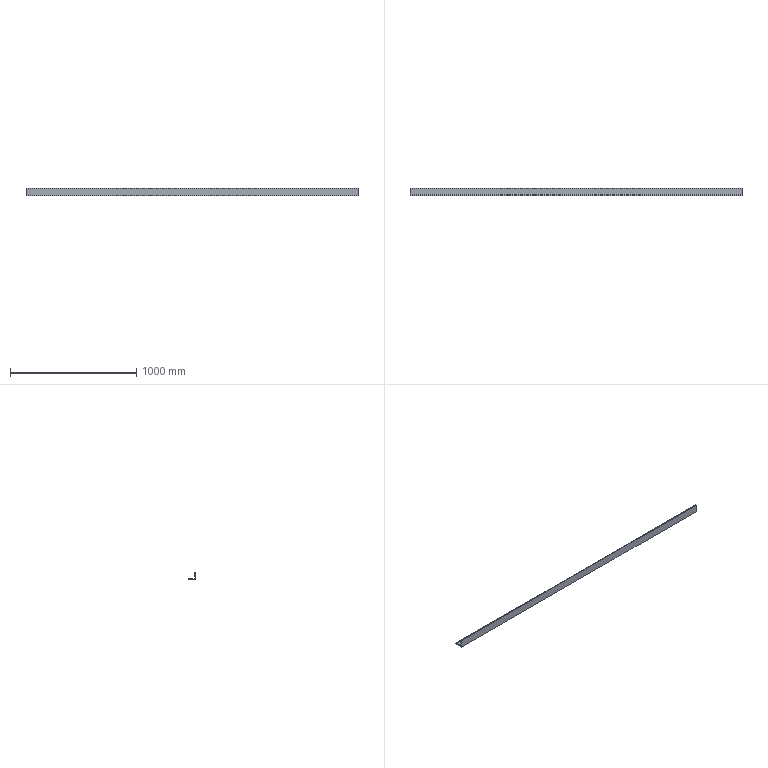Part | STEP file | Angle steel L63X63X8-2626_Default<As machined> | 1 solid | 11 faces | box 2626 x 63 x 63 mm | volume 2498543 mm3 | plane 8 | cylinder 3 | commonest cylinder face diameters 5.333 x2 14 x1
STEP:
#1=CARTESIAN_POINT('',(0.,0.,0.));
#2=DIRECTION('',(0.,0.,1.));
#3=DIRECTION('',(1.,0.,0.));
#4=AXIS2_PLACEMENT_3D('',#1,#2,#3);
#5=CARTESIAN_POINT('',(-1313.,0.,0.));
#6=VERTEX_POINT('',#5);
#7=CARTESIAN_POINT('',(-1313.,63.,0.));
#8=VERTEX_POINT('',#7);
#9=CARTESIAN_POINT('',(-1313.,63.,0.));
#10=DIRECTION('',(0.,1.,0.));
#11=VECTOR('',#10,1.);
#12=LINE('',#9,#11);
#13=CARTESIAN_POINT('',(1313.,63.,0.));
#14=DIRECTION('',(0.,0.,1.));
#15=DIRECTION('',(1.,0.,0.));
#16=AXIS2_PLACEMENT_3D('',#13,#14,#15);
#17=PLANE('',#16);
#18=CARTESIAN_POINT('',(-2626.,0.));
#19=DIRECTION('',(0.,1.));
#20=VECTOR('',#19,1.);
#21=LINE('',#18,#20);
#22=(GEOMETRIC_REPRESENTATION_CONTEXT(2)PARAMETRIC_REPRESENTATION_CONTEXT()REPRESENTATION_CONTEXT('',''));
#23=DEFINITIONAL_REPRESENTATION('',(#21),#22);
#24=PCURVE('',#17,#23);
#25=CARTESIAN_POINT('',(-1313.,5.333,60.333));
#26=DIRECTION('',(-1.,0.,0.));
#27=DIRECTION('',(0.,0.,1.));
#28=AXIS2_PLACEMENT_3D('',#25,#26,#27);
#29=PLANE('',#28);
#30=CARTESIAN_POINT('',(-60.333,57.667));
#31=DIRECTION('',(0.,1.));
#32=VECTOR('',#31,1.);
#33=LINE('',#30,#32);
#34=(GEOMETRIC_REPRESENTATION_CONTEXT(2)PARAMETRIC_REPRESENTATION_CONTEXT()REPRESENTATION_CONTEXT('',''));
#35=DEFINITIONAL_REPRESENTATION('',(#33),#34);
#36=PCURVE('',#29,#35);
#37=SURFACE_CURVE('',#12,(#24,#36),.PCURVE_S1.);
#38=EDGE_CURVE('',#6,#8,#37,.T.);
#39=ORIENTED_EDGE('',*,*,#38,.T.);
#40=CARTESIAN_POINT('',(1313.,63.,0.));
#41=VERTEX_POINT('',#40);
#42=CARTESIAN_POINT('',(1313.,63.,0.));
#43=DIRECTION('',(-1.,0.,0.));
#44=VECTOR('',#43,1.);
#45=LINE('',#42,#44);
#46=CARTESIAN_POINT('',(0.,0.));
#47=DIRECTION('',(-1.,0.));
#48=VECTOR('',#47,1.);
#49=LINE('',#46,#48);
#50=(GEOMETRIC_REPRESENTATION_CONTEXT(2)PARAMETRIC_REPRESENTATION_CONTEXT()REPRESENTATION_CONTEXT('',''));
#51=DEFINITIONAL_REPRESENTATION('',(#49),#50);
#52=PCURVE('',#17,#51);
#53=CARTESIAN_POINT('',(1313.,63.,0.));
#54=DIRECTION('',(0.,-1.,0.));
#55=DIRECTION('',(0.,0.,-1.));
#56=AXIS2_PLACEMENT_3D('',#53,#54,#55);
#57=PLANE('',#56);
#58=CARTESIAN_POINT('',(0.,0.));
#59=DIRECTION('',(0.,-1.));
#60=VECTOR('',#59,1.);
#61=LINE('',#58,#60);
#62=(GEOMETRIC_REPRESENTATION_CONTEXT(2)PARAMETRIC_REPRESENTATION_CONTEXT()REPRESENTATION_CONTEXT('',''));
#63=DEFINITIONAL_REPRESENTATION('',(#61),#62);
#64=PCURVE('',#57,#63);
#65=SURFACE_CURVE('',#45,(#52,#64),.PCURVE_S1.);
#66=EDGE_CURVE('',#41,#8,#65,.T.);
#67=ORIENTED_EDGE('',*,*,#66,.F.);
#68=CARTESIAN_POINT('',(1313.,0.,0.));
#69=VERTEX_POINT('',#68);
#70=CARTESIAN_POINT('',(1313.,63.,0.));
#71=DIRECTION('',(0.,1.,0.));
#72=VECTOR('',#71,1.);
#73=LINE('',#70,#72);
#74=CARTESIAN_POINT('',(0.,0.));
#75=DIRECTION('',(0.,1.));
#76=VECTOR('',#75,1.);
#77=LINE('',#74,#76);
#78=(GEOMETRIC_REPRESENTATION_CONTEXT(2)PARAMETRIC_REPRESENTATION_CONTEXT()REPRESENTATION_CONTEXT('',''));
#79=DEFINITIONAL_REPRESENTATION('',(#77),#78);
#80=PCURVE('',#17,#79);
#81=CARTESIAN_POINT('',(1313.,5.333,60.333));
#82=DIRECTION('',(-1.,0.,0.));
#83=DIRECTION('',(0.,0.,1.));
#84=AXIS2_PLACEMENT_3D('',#81,#82,#83);
#85=PLANE('',#84);
#86=CARTESIAN_POINT('',(-60.333,57.667));
#87=DIRECTION('',(0.,1.));
#88=VECTOR('',#87,1.);
#89=LINE('',#86,#88);
#90=(GEOMETRIC_REPRESENTATION_CONTEXT(2)PARAMETRIC_REPRESENTATION_CONTEXT()REPRESENTATION_CONTEXT('',''));
#91=DEFINITIONAL_REPRESENTATION('',(#89),#90);
#92=PCURVE('',#85,#91);
#93=SURFACE_CURVE('',#73,(#80,#92),.PCURVE_S1.);
#94=EDGE_CURVE('',#69,#41,#93,.T.);
#95=ORIENTED_EDGE('',*,*,#94,.F.);
#96=CARTESIAN_POINT('',(1313.,0.,0.));
#97=DIRECTION('',(-1.,0.,0.));
#98=VECTOR('',#97,1.);
#99=LINE('',#96,#98);
#100=CARTESIAN_POINT('',(0.,-63.));
#101=DIRECTION('',(-1.,0.));
#102=VECTOR('',#101,1.);
#103=LINE('',#100,#102);
#104=(GEOMETRIC_REPRESENTATION_CONTEXT(2)PARAMETRIC_REPRESENTATION_CONTEXT()REPRESENTATION_CONTEXT('',''));
#105=DEFINITIONAL_REPRESENTATION('',(#103),#104);
#106=PCURVE('',#17,#105);
#107=CARTESIAN_POINT('',(1313.,0.,0.));
#108=DIRECTION('',(0.,1.,0.));
#109=DIRECTION('',(0.,0.,1.));
#110=AXIS2_PLACEMENT_3D('',#107,#108,#109);
#111=PLANE('',#110);
#112=CARTESIAN_POINT('',(0.,0.));
#113=DIRECTION('',(0.,-1.));
#114=VECTOR('',#113,1.);
#115=LINE('',#112,#114);
#116=(GEOMETRIC_REPRESENTATION_CONTEXT(2)PARAMETRIC_REPRESENTATION_CONTEXT()REPRESENTATION_CONTEXT('',''));
#117=DEFINITIONAL_REPRESENTATION('',(#115),#116);
#118=PCURVE('',#111,#117);
#119=SURFACE_CURVE('',#99,(#106,#118),.PCURVE_S1.);
#120=EDGE_CURVE('',#69,#6,#119,.T.);
#121=ORIENTED_EDGE('',*,*,#120,.T.);
#122=EDGE_LOOP('',(#39,#67,#95,#121));
#123=FACE_BOUND('',#122,.T.);
#124=ADVANCED_FACE('',(#123),#17,.F.);
#125=CARTESIAN_POINT('',(-1313.,63.,5.333));
#126=VERTEX_POINT('',#125);
#127=CARTESIAN_POINT('',(-1313.,63.,0.));
#128=DIRECTION('',(0.,0.,1.));
#129=VECTOR('',#128,1.);
#130=LINE('',#127,#129);
#131=CARTESIAN_POINT('',(0.,-2626.));
#132=DIRECTION('',(-1.,0.));
#133=VECTOR('',#132,1.);
#134=LINE('',#131,#133);
#135=(GEOMETRIC_REPRESENTATION_CONTEXT(2)PARAMETRIC_REPRESENTATION_CONTEXT()REPRESENTATION_CONTEXT('',''));
#136=DEFINITIONAL_REPRESENTATION('',(#134),#135);
#137=PCURVE('',#57,#136);
#138=CARTESIAN_POINT('',(-60.333,57.667));
#139=DIRECTION('',(1.,0.));
#140=VECTOR('',#139,1.);
#141=LINE('',#138,#140);
#142=(GEOMETRIC_REPRESENTATION_CONTEXT(2)PARAMETRIC_REPRESENTATION_CONTEXT()REPRESENTATION_CONTEXT('',''));
#143=DEFINITIONAL_REPRESENTATION('',(#141),#142);
#144=PCURVE('',#29,#143);
#145=SURFACE_CURVE('',#130,(#137,#144),.PCURVE_S1.);
#146=EDGE_CURVE('',#8,#126,#145,.T.);
#147=ORIENTED_EDGE('',*,*,#146,.T.);
#148=CARTESIAN_POINT('',(1313.,63.,5.333));
#149=VERTEX_POINT('',#148);
#150=CARTESIAN_POINT('',(1313.,63.,5.333));
#151=DIRECTION('',(-1.,0.,0.));
#152=VECTOR('',#151,1.);
#153=LINE('',#150,#152);
#154=CARTESIAN_POINT('',(-5.333,0.));
#155=DIRECTION('',(0.,-1.));
#156=VECTOR('',#155,1.);
#157=LINE('',#154,#156);
#158=(GEOMETRIC_REPRESENTATION_CONTEXT(2)PARAMETRIC_REPRESENTATION_CONTEXT()REPRESENTATION_CONTEXT('',''));
#159=DEFINITIONAL_REPRESENTATION('',(#157),#158);
#160=PCURVE('',#57,#159);
#161=CARTESIAN_POINT('',(1313.,60.333,5.333));
#162=DIRECTION('',(-1.,0.,0.));
#163=DIRECTION('',(0.,0.,1.));
#164=AXIS2_PLACEMENT_3D('',#161,#162,#163);
#165=CYLINDRICAL_SURFACE('',#164,2.667);
#166=CARTESIAN_POINT('',(1.571,0.));
#167=DIRECTION('',(0.,1.));
#168=VECTOR('',#167,1.);
#169=LINE('',#166,#168);
#170=(GEOMETRIC_REPRESENTATION_CONTEXT(2)PARAMETRIC_REPRESENTATION_CONTEXT()REPRESENTATION_CONTEXT('',''));
#171=DEFINITIONAL_REPRESENTATION('',(#169),#170);
#172=PCURVE('',#165,#171);
#173=SURFACE_CURVE('',#153,(#160,#172),.PCURVE_S1.);
#174=EDGE_CURVE('',#149,#126,#173,.T.);
#175=ORIENTED_EDGE('',*,*,#174,.F.);
#176=CARTESIAN_POINT('',(1313.,63.,0.));
#177=DIRECTION('',(0.,0.,1.));
#178=VECTOR('',#177,1.);
#179=LINE('',#176,#178);
#180=CARTESIAN_POINT('',(0.,0.));
#181=DIRECTION('',(-1.,0.));
#182=VECTOR('',#181,1.);
#183=LINE('',#180,#182);
#184=(GEOMETRIC_REPRESENTATION_CONTEXT(2)PARAMETRIC_REPRESENTATION_CONTEXT()REPRESENTATION_CONTEXT('',''));
#185=DEFINITIONAL_REPRESENTATION('',(#183),#184);
#186=PCURVE('',#57,#185);
#187=CARTESIAN_POINT('',(-60.333,57.667));
#188=DIRECTION('',(1.,0.));
#189=VECTOR('',#188,1.);
#190=LINE('',#187,#189);
#191=(GEOMETRIC_REPRESENTATION_CONTEXT(2)PARAMETRIC_REPRESENTATION_CONTEXT()REPRESENTATION_CONTEXT('',''));
#192=DEFINITIONAL_REPRESENTATION('',(#190),#191);
#193=PCURVE('',#85,#192);
#194=SURFACE_CURVE('',#179,(#186,#193),.PCURVE_S1.);
#195=EDGE_CURVE('',#41,#149,#194,.T.);
#196=ORIENTED_EDGE('',*,*,#195,.F.);
#197=ORIENTED_EDGE('',*,*,#66,.T.);
#198=EDGE_LOOP('',(#147,#175,#196,#197));
#199=FACE_BOUND('',#198,.T.);
#200=ADVANCED_FACE('',(#199),#57,.F.);
#201=CARTESIAN_POINT('',(-1313.,60.333,8.));
#202=VERTEX_POINT('',#201);
#203=CARTESIAN_POINT('',(-1313.,60.333,5.333));
#204=DIRECTION('',(1.,0.,0.));
#205=DIRECTION('',(0.,0.,-1.));
#206=AXIS2_PLACEMENT_3D('',#203,#204,#205);
#207=CIRCLE('',#206,2.667);
#208=CARTESIAN_POINT('',(3.142,2626.));
#209=DIRECTION('',(-1.,0.));
#210=VECTOR('',#209,1.);
#211=LINE('',#208,#210);
#212=(GEOMETRIC_REPRESENTATION_CONTEXT(2)PARAMETRIC_REPRESENTATION_CONTEXT()REPRESENTATION_CONTEXT('',''));
#213=DEFINITIONAL_REPRESENTATION('',(#211),#212);
#214=PCURVE('',#165,#213);
#215=CARTESIAN_POINT('',(-57.667,55.));
#216=CARTESIAN_POINT('',(-57.667,59.619));
#217=CARTESIAN_POINT('',(-53.667,57.309));
#218=CARTESIAN_POINT('',(-49.667,55.));
#219=CARTESIAN_POINT('',(-53.667,52.691));
#220=CARTESIAN_POINT('',(-57.667,50.381));
#221=CARTESIAN_POINT('',(-57.667,55.));
#222=(BOUNDED_CURVE()B_SPLINE_CURVE(2,(#215,#216,#217,#218,#219,#220,#221),.UNSPECIFIED.,.T.,.F.)B_SPLINE_CURVE_WITH_KNOTS((1,2,2,2,2,1),(-2.094,0.,2.094,4.189,6.283,8.378),.UNSPECIFIED.)CURVE()GEOMETRIC_REPRESENTATION_ITEM()RATIONAL_B_SPLINE_CURVE((1.,0.5,1.,0.5,1.,0.5,1.))REPRESENTATION_ITEM(''));
#223=(GEOMETRIC_REPRESENTATION_CONTEXT(2)PARAMETRIC_REPRESENTATION_CONTEXT()REPRESENTATION_CONTEXT('',''));
#224=DEFINITIONAL_REPRESENTATION('',(#222),#223);
#225=PCURVE('',#29,#224);
#226=SURFACE_CURVE('',#207,(#214,#225),.PCURVE_S1.);
#227=EDGE_CURVE('',#126,#202,#226,.T.);
#228=ORIENTED_EDGE('',*,*,#227,.T.);
#229=CARTESIAN_POINT('',(1313.,60.333,8.));
#230=VERTEX_POINT('',#229);
#231=CARTESIAN_POINT('',(1313.,60.333,8.));
#232=DIRECTION('',(-1.,0.,0.));
#233=VECTOR('',#232,1.);
#234=LINE('',#231,#233);
#235=CARTESIAN_POINT('',(0.,0.));
#236=DIRECTION('',(0.,1.));
#237=VECTOR('',#236,1.);
#238=LINE('',#235,#237);
#239=(GEOMETRIC_REPRESENTATION_CONTEXT(2)PARAMETRIC_REPRESENTATION_CONTEXT()REPRESENTATION_CONTEXT('',''));
#240=DEFINITIONAL_REPRESENTATION('',(#238),#239);
#241=PCURVE('',#165,#240);
#242=CARTESIAN_POINT('',(1313.,15.,8.));
#243=DIRECTION('',(0.,0.,-1.));
#244=DIRECTION('',(-1.,0.,0.));
#245=AXIS2_PLACEMENT_3D('',#242,#243,#244);
#246=PLANE('',#245);
#247=CARTESIAN_POINT('',(0.,45.333));
#248=DIRECTION('',(1.,0.));
#249=VECTOR('',#248,1.);
#250=LINE('',#247,#249);
#251=(GEOMETRIC_REPRESENTATION_CONTEXT(2)PARAMETRIC_REPRESENTATION_CONTEXT()REPRESENTATION_CONTEXT('',''));
#252=DEFINITIONAL_REPRESENTATION('',(#250),#251);
#253=PCURVE('',#246,#252);
#254=SURFACE_CURVE('',#234,(#241,#253),.PCURVE_S1.);
#255=EDGE_CURVE('',#230,#202,#254,.T.);
#256=ORIENTED_EDGE('',*,*,#255,.F.);
#257=CARTESIAN_POINT('',(1313.,60.333,5.333));
#258=DIRECTION('',(1.,0.,0.));
#259=DIRECTION('',(0.,0.,-1.));
#260=AXIS2_PLACEMENT_3D('',#257,#258,#259);
#261=CIRCLE('',#260,2.667);
#262=CARTESIAN_POINT('',(3.142,0.));
#263=DIRECTION('',(-1.,0.));
#264=VECTOR('',#263,1.);
#265=LINE('',#262,#264);
#266=(GEOMETRIC_REPRESENTATION_CONTEXT(2)PARAMETRIC_REPRESENTATION_CONTEXT()REPRESENTATION_CONTEXT('',''));
#267=DEFINITIONAL_REPRESENTATION('',(#265),#266);
#268=PCURVE('',#165,#267);
#269=CARTESIAN_POINT('',(-57.667,55.));
#270=CARTESIAN_POINT('',(-57.667,59.619));
#271=CARTESIAN_POINT('',(-53.667,57.309));
#272=CARTESIAN_POINT('',(-49.667,55.));
#273=CARTESIAN_POINT('',(-53.667,52.691));
#274=CARTESIAN_POINT('',(-57.667,50.381));
#275=CARTESIAN_POINT('',(-57.667,55.));
#276=(BOUNDED_CURVE()B_SPLINE_CURVE(2,(#269,#270,#271,#272,#273,#274,#275),.UNSPECIFIED.,.T.,.F.)B_SPLINE_CURVE_WITH_KNOTS((1,2,2,2,2,1),(-2.094,0.,2.094,4.189,6.283,8.378),.UNSPECIFIED.)CURVE()GEOMETRIC_REPRESENTATION_ITEM()RATIONAL_B_SPLINE_CURVE((1.,0.5,1.,0.5,1.,0.5,1.))REPRESENTATION_ITEM(''));
#277=(GEOMETRIC_REPRESENTATION_CONTEXT(2)PARAMETRIC_REPRESENTATION_CONTEXT()REPRESENTATION_CONTEXT('',''));
#278=DEFINITIONAL_REPRESENTATION('',(#276),#277);
#279=PCURVE('',#85,#278);
#280=SURFACE_CURVE('',#261,(#268,#279),.PCURVE_S1.);
#281=EDGE_CURVE('',#149,#230,#280,.T.);
#282=ORIENTED_EDGE('',*,*,#281,.F.);
#283=ORIENTED_EDGE('',*,*,#174,.T.);
#284=EDGE_LOOP('',(#228,#256,#282,#283));
#285=FACE_BOUND('',#284,.T.);
#286=ADVANCED_FACE('',(#285),#165,.T.);
#287=CARTESIAN_POINT('',(-1313.,15.,8.));
#288=VERTEX_POINT('',#287);
#289=CARTESIAN_POINT('',(-1313.,15.,8.));
#290=DIRECTION('',(0.,-1.,0.));
#291=VECTOR('',#290,1.);
#292=LINE('',#289,#291);
#293=CARTESIAN_POINT('',(2626.,0.));
#294=DIRECTION('',(0.,-1.));
#295=VECTOR('',#294,1.);
#296=LINE('',#293,#295);
#297=(GEOMETRIC_REPRESENTATION_CONTEXT(2)PARAMETRIC_REPRESENTATION_CONTEXT()REPRESENTATION_CONTEXT('',''));
#298=DEFINITIONAL_REPRESENTATION('',(#296),#297);
#299=PCURVE('',#246,#298);
#300=CARTESIAN_POINT('',(-52.333,9.667));
#301=DIRECTION('',(0.,-1.));
#302=VECTOR('',#301,1.);
#303=LINE('',#300,#302);
#304=(GEOMETRIC_REPRESENTATION_CONTEXT(2)PARAMETRIC_REPRESENTATION_CONTEXT()REPRESENTATION_CONTEXT('',''));
#305=DEFINITIONAL_REPRESENTATION('',(#303),#304);
#306=PCURVE('',#29,#305);
#307=SURFACE_CURVE('',#292,(#299,#306),.PCURVE_S1.);
#308=EDGE_CURVE('',#202,#288,#307,.T.);
#309=ORIENTED_EDGE('',*,*,#308,.T.);
#310=CARTESIAN_POINT('',(1313.,15.,8.));
#311=VERTEX_POINT('',#310);
#312=CARTESIAN_POINT('',(1313.,15.,8.));
#313=DIRECTION('',(-1.,0.,0.));
#314=VECTOR('',#313,1.);
#315=LINE('',#312,#314);
#316=CARTESIAN_POINT('',(0.,0.));
#317=DIRECTION('',(1.,0.));
#318=VECTOR('',#317,1.);
#319=LINE('',#316,#318);
#320=(GEOMETRIC_REPRESENTATION_CONTEXT(2)PARAMETRIC_REPRESENTATION_CONTEXT()REPRESENTATION_CONTEXT('',''));
#321=DEFINITIONAL_REPRESENTATION('',(#319),#320);
#322=PCURVE('',#246,#321);
#323=CARTESIAN_POINT('',(1313.,15.,15.));
#324=DIRECTION('',(-1.,0.,0.));
#325=DIRECTION('',(0.,0.,1.));
#326=AXIS2_PLACEMENT_3D('',#323,#324,#325);
#327=CYLINDRICAL_SURFACE('',#326,7.);
#328=CARTESIAN_POINT('',(3.142,0.));
#329=DIRECTION('',(0.,1.));
#330=VECTOR('',#329,1.);
#331=LINE('',#328,#330);
#332=(GEOMETRIC_REPRESENTATION_CONTEXT(2)PARAMETRIC_REPRESENTATION_CONTEXT()REPRESENTATION_CONTEXT('',''));
#333=DEFINITIONAL_REPRESENTATION('',(#331),#332);
#334=PCURVE('',#327,#333);
#335=SURFACE_CURVE('',#315,(#322,#334),.PCURVE_S1.);
#336=EDGE_CURVE('',#311,#288,#335,.T.);
#337=ORIENTED_EDGE('',*,*,#336,.F.);
#338=CARTESIAN_POINT('',(1313.,15.,8.));
#339=DIRECTION('',(0.,-1.,0.));
#340=VECTOR('',#339,1.);
#341=LINE('',#338,#340);
#342=CARTESIAN_POINT('',(0.,0.));
#343=DIRECTION('',(0.,-1.));
#344=VECTOR('',#343,1.);
#345=LINE('',#342,#344);
#346=(GEOMETRIC_REPRESENTATION_CONTEXT(2)PARAMETRIC_REPRESENTATION_CONTEXT()REPRESENTATION_CONTEXT('',''));
#347=DEFINITIONAL_REPRESENTATION('',(#345),#346);
#348=PCURVE('',#246,#347);
#349=CARTESIAN_POINT('',(-52.333,9.667));
#350=DIRECTION('',(0.,-1.));
#351=VECTOR('',#350,1.);
#352=LINE('',#349,#351);
#353=(GEOMETRIC_REPRESENTATION_CONTEXT(2)PARAMETRIC_REPRESENTATION_CONTEXT()REPRESENTATION_CONTEXT('',''));
#354=DEFINITIONAL_REPRESENTATION('',(#352),#353);
#355=PCURVE('',#85,#354);
#356=SURFACE_CURVE('',#341,(#348,#355),.PCURVE_S1.);
#357=EDGE_CURVE('',#230,#311,#356,.T.);
#358=ORIENTED_EDGE('',*,*,#357,.F.);
#359=ORIENTED_EDGE('',*,*,#255,.T.);
#360=EDGE_LOOP('',(#309,#337,#358,#359));
#361=FACE_BOUND('',#360,.T.);
#362=ADVANCED_FACE('',(#361),#246,.F.);
#363=ORIENTED_EDGE('',*,*,#336,.F.);
#364=CARTESIAN_POINT('',(1313.,8.,15.));
#365=VERTEX_POINT('',#364);
#366=CARTESIAN_POINT('',(1313.,15.,15.));
#367=DIRECTION('',(-1.,0.,0.));
#368=DIRECTION('',(0.,0.,1.));
#369=AXIS2_PLACEMENT_3D('',#366,#367,#368);
#370=CIRCLE('',#369,7.);
#371=CARTESIAN_POINT('',(0.,0.));
#372=DIRECTION('',(1.,0.));
#373=VECTOR('',#372,1.);
#374=LINE('',#371,#373);
#375=(GEOMETRIC_REPRESENTATION_CONTEXT(2)PARAMETRIC_REPRESENTATION_CONTEXT()REPRESENTATION_CONTEXT('',''));
#376=DEFINITIONAL_REPRESENTATION('',(#374),#375);
#377=PCURVE('',#327,#376);
#378=CARTESIAN_POINT('',(-45.333,9.667));
#379=DIRECTION('',(1.,0.));
#380=AXIS2_PLACEMENT_2D('',#378,#379);
#381=CIRCLE('',#380,7.);
#382=(GEOMETRIC_REPRESENTATION_CONTEXT(2)PARAMETRIC_REPRESENTATION_CONTEXT()REPRESENTATION_CONTEXT('',''));
#383=DEFINITIONAL_REPRESENTATION('',(#381),#382);
#384=PCURVE('',#85,#383);
#385=SURFACE_CURVE('',#370,(#377,#384),.PCURVE_S1.);
#386=EDGE_CURVE('',#311,#365,#385,.T.);
#387=ORIENTED_EDGE('',*,*,#386,.T.);
#388=CARTESIAN_POINT('',(-1313.,8.,15.));
#389=VERTEX_POINT('',#388);
#390=CARTESIAN_POINT('',(1313.,8.,15.));
#391=DIRECTION('',(-1.,0.,0.));
#392=VECTOR('',#391,1.);
#393=LINE('',#390,#392);
#394=CARTESIAN_POINT('',(4.712,0.));
#395=DIRECTION('',(0.,1.));
#396=VECTOR('',#395,1.);
#397=LINE('',#394,#396);
#398=(GEOMETRIC_REPRESENTATION_CONTEXT(2)PARAMETRIC_REPRESENTATION_CONTEXT()REPRESENTATION_CONTEXT('',''));
#399=DEFINITIONAL_REPRESENTATION('',(#397),#398);
#400=PCURVE('',#327,#399);
#401=CARTESIAN_POINT('',(1313.,8.,60.333));
#402=DIRECTION('',(0.,-1.,0.));
#403=DIRECTION('',(0.,0.,-1.));
#404=AXIS2_PLACEMENT_3D('',#401,#402,#403);
#405=PLANE('',#404);
#406=CARTESIAN_POINT('',(45.333,0.));
#407=DIRECTION('',(0.,-1.));
#408=VECTOR('',#407,1.);
#409=LINE('',#406,#408);
#410=(GEOMETRIC_REPRESENTATION_CONTEXT(2)PARAMETRIC_REPRESENTATION_CONTEXT()REPRESENTATION_CONTEXT('',''));
#411=DEFINITIONAL_REPRESENTATION('',(#409),#410);
#412=PCURVE('',#405,#411);
#413=SURFACE_CURVE('',#393,(#400,#412),.PCURVE_S1.);
#414=EDGE_CURVE('',#365,#389,#413,.T.);
#415=ORIENTED_EDGE('',*,*,#414,.T.);
#416=CARTESIAN_POINT('',(-1313.,15.,15.));
#417=DIRECTION('',(-1.,0.,0.));
#418=DIRECTION('',(0.,0.,1.));
#419=AXIS2_PLACEMENT_3D('',#416,#417,#418);
#420=CIRCLE('',#419,7.);
#421=CARTESIAN_POINT('',(0.,2626.));
#422=DIRECTION('',(1.,0.));
#423=VECTOR('',#422,1.);
#424=LINE('',#421,#423);
#425=(GEOMETRIC_REPRESENTATION_CONTEXT(2)PARAMETRIC_REPRESENTATION_CONTEXT()REPRESENTATION_CONTEXT('',''));
#426=DEFINITIONAL_REPRESENTATION('',(#424),#425);
#427=PCURVE('',#327,#426);
#428=CARTESIAN_POINT('',(-45.333,9.667));
#429=DIRECTION('',(1.,0.));
#430=AXIS2_PLACEMENT_2D('',#428,#429);
#431=CIRCLE('',#430,7.);
#432=(GEOMETRIC_REPRESENTATION_CONTEXT(2)PARAMETRIC_REPRESENTATION_CONTEXT()REPRESENTATION_CONTEXT('',''));
#433=DEFINITIONAL_REPRESENTATION('',(#431),#432);
#434=PCURVE('',#29,#433);
#435=SURFACE_CURVE('',#420,(#427,#434),.PCURVE_S1.);
#436=EDGE_CURVE('',#288,#389,#435,.T.);
#437=ORIENTED_EDGE('',*,*,#436,.F.);
#438=EDGE_LOOP('',(#363,#387,#415,#437));
#439=FACE_BOUND('',#438,.F.);
#440=ADVANCED_FACE('',(#439),#327,.F.);
#441=CARTESIAN_POINT('',(-1313.,8.,60.333));
#442=VERTEX_POINT('',#441);
#443=CARTESIAN_POINT('',(-1313.,8.,60.333));
#444=DIRECTION('',(0.,0.,1.));
#445=VECTOR('',#444,1.);
#446=LINE('',#443,#445);
#447=CARTESIAN_POINT('',(0.,-2626.));
#448=DIRECTION('',(-1.,0.));
#449=VECTOR('',#448,1.);
#450=LINE('',#447,#449);
#451=(GEOMETRIC_REPRESENTATION_CONTEXT(2)PARAMETRIC_REPRESENTATION_CONTEXT()REPRESENTATION_CONTEXT('',''));
#452=DEFINITIONAL_REPRESENTATION('',(#450),#451);
#453=PCURVE('',#405,#452);
#454=CARTESIAN_POINT('',(0.,2.667));
#455=DIRECTION('',(1.,0.));
#456=VECTOR('',#455,1.);
#457=LINE('',#454,#456);
#458=(GEOMETRIC_REPRESENTATION_CONTEXT(2)PARAMETRIC_REPRESENTATION_CONTEXT()REPRESENTATION_CONTEXT('',''));
#459=DEFINITIONAL_REPRESENTATION('',(#457),#458);
#460=PCURVE('',#29,#459);
#461=SURFACE_CURVE('',#446,(#453,#460),.PCURVE_S1.);
#462=EDGE_CURVE('',#389,#442,#461,.T.);
#463=ORIENTED_EDGE('',*,*,#462,.T.);
#464=CARTESIAN_POINT('',(1313.,8.,60.333));
#465=VERTEX_POINT('',#464);
#466=CARTESIAN_POINT('',(1313.,8.,60.333));
#467=DIRECTION('',(-1.,0.,0.));
#468=VECTOR('',#467,1.);
#469=LINE('',#466,#468);
#470=CARTESIAN_POINT('',(0.,0.));
#471=DIRECTION('',(0.,-1.));
#472=VECTOR('',#471,1.);
#473=LINE('',#470,#472);
#474=(GEOMETRIC_REPRESENTATION_CONTEXT(2)PARAMETRIC_REPRESENTATION_CONTEXT()REPRESENTATION_CONTEXT('',''));
#475=DEFINITIONAL_REPRESENTATION('',(#473),#474);
#476=PCURVE('',#405,#475);
#477=CARTESIAN_POINT('',(1313.,5.333,60.333));
#478=DIRECTION('',(-1.,0.,0.));
#479=DIRECTION('',(0.,0.,1.));
#480=AXIS2_PLACEMENT_3D('',#477,#478,#479);
#481=CYLINDRICAL_SURFACE('',#480,2.667);
#482=CARTESIAN_POINT('',(1.571,0.));
#483=DIRECTION('',(0.,1.));
#484=VECTOR('',#483,1.);
#485=LINE('',#482,#484);
#486=(GEOMETRIC_REPRESENTATION_CONTEXT(2)PARAMETRIC_REPRESENTATION_CONTEXT()REPRESENTATION_CONTEXT('',''));
#487=DEFINITIONAL_REPRESENTATION('',(#485),#486);
#488=PCURVE('',#481,#487);
#489=SURFACE_CURVE('',#469,(#476,#488),.PCURVE_S1.);
#490=EDGE_CURVE('',#465,#442,#489,.T.);
#491=ORIENTED_EDGE('',*,*,#490,.F.);
#492=CARTESIAN_POINT('',(1313.,8.,60.333));
#493=DIRECTION('',(0.,0.,1.));
#494=VECTOR('',#493,1.);
#495=LINE('',#492,#494);
#496=CARTESIAN_POINT('',(0.,0.));
#497=DIRECTION('',(-1.,0.));
#498=VECTOR('',#497,1.);
#499=LINE('',#496,#498);
#500=(GEOMETRIC_REPRESENTATION_CONTEXT(2)PARAMETRIC_REPRESENTATION_CONTEXT()REPRESENTATION_CONTEXT('',''));
#501=DEFINITIONAL_REPRESENTATION('',(#499),#500);
#502=PCURVE('',#405,#501);
#503=CARTESIAN_POINT('',(0.,2.667));
#504=DIRECTION('',(1.,0.));
#505=VECTOR('',#504,1.);
#506=LINE('',#503,#505);
#507=(GEOMETRIC_REPRESENTATION_CONTEXT(2)PARAMETRIC_REPRESENTATION_CONTEXT()REPRESENTATION_CONTEXT('',''));
#508=DEFINITIONAL_REPRESENTATION('',(#506),#507);
#509=PCURVE('',#85,#508);
#510=SURFACE_CURVE('',#495,(#502,#509),.PCURVE_S1.);
#511=EDGE_CURVE('',#365,#465,#510,.T.);
#512=ORIENTED_EDGE('',*,*,#511,.F.);
#513=ORIENTED_EDGE('',*,*,#414,.T.);
#514=EDGE_LOOP('',(#463,#491,#512,#513));
#515=FACE_BOUND('',#514,.T.);
#516=ADVANCED_FACE('',(#515),#405,.F.);
#517=CARTESIAN_POINT('',(-1313.,5.333,63.));
#518=VERTEX_POINT('',#517);
#519=CARTESIAN_POINT('',(-1313.,5.333,60.333));
#520=DIRECTION('',(1.,0.,0.));
#521=DIRECTION('',(0.,0.,1.));
#522=AXIS2_PLACEMENT_3D('',#519,#520,#521);
#523=CIRCLE('',#522,2.667);
#524=CARTESIAN_POINT('',(6.283,2626.));
#525=DIRECTION('',(-1.,0.));
#526=VECTOR('',#525,1.);
#527=LINE('',#524,#526);
#528=(GEOMETRIC_REPRESENTATION_CONTEXT(2)PARAMETRIC_REPRESENTATION_CONTEXT()REPRESENTATION_CONTEXT('',''));
#529=DEFINITIONAL_REPRESENTATION('',(#527),#528);
#530=PCURVE('',#481,#529);
#531=CARTESIAN_POINT('',(2.667,0.));
#532=CARTESIAN_POINT('',(2.667,-4.619));
#533=CARTESIAN_POINT('',(-1.333,-2.309));
#534=CARTESIAN_POINT('',(-5.333,0.));
#535=CARTESIAN_POINT('',(-1.333,2.309));
#536=CARTESIAN_POINT('',(2.667,4.619));
#537=CARTESIAN_POINT('',(2.667,0.));
#538=(BOUNDED_CURVE()B_SPLINE_CURVE(2,(#531,#532,#533,#534,#535,#536,#537),.UNSPECIFIED.,.T.,.F.)B_SPLINE_CURVE_WITH_KNOTS((1,2,2,2,2,1),(-2.094,0.,2.094,4.189,6.283,8.378),.UNSPECIFIED.)CURVE()GEOMETRIC_REPRESENTATION_ITEM()RATIONAL_B_SPLINE_CURVE((1.,0.5,1.,0.5,1.,0.5,1.))REPRESENTATION_ITEM(''));
#539=(GEOMETRIC_REPRESENTATION_CONTEXT(2)PARAMETRIC_REPRESENTATION_CONTEXT()REPRESENTATION_CONTEXT('',''));
#540=DEFINITIONAL_REPRESENTATION('',(#538),#539);
#541=PCURVE('',#29,#540);
#542=SURFACE_CURVE('',#523,(#530,#541),.PCURVE_S1.);
#543=EDGE_CURVE('',#442,#518,#542,.T.);
#544=ORIENTED_EDGE('',*,*,#543,.T.);
#545=CARTESIAN_POINT('',(1313.,5.333,63.));
#546=VERTEX_POINT('',#545);
#547=CARTESIAN_POINT('',(1313.,5.333,63.));
#548=DIRECTION('',(-1.,0.,0.));
#549=VECTOR('',#548,1.);
#550=LINE('',#547,#549);
#551=CARTESIAN_POINT('',(0.,0.));
#552=DIRECTION('',(0.,1.));
#553=VECTOR('',#552,1.);
#554=LINE('',#551,#553);
#555=(GEOMETRIC_REPRESENTATION_CONTEXT(2)PARAMETRIC_REPRESENTATION_CONTEXT()REPRESENTATION_CONTEXT('',''));
#556=DEFINITIONAL_REPRESENTATION('',(#554),#555);
#557=PCURVE('',#481,#556);
#558=CARTESIAN_POINT('',(1313.,0.,63.));
#559=DIRECTION('',(0.,0.,-1.));
#560=DIRECTION('',(0.,1.,0.));
#561=AXIS2_PLACEMENT_3D('',#558,#559,#560);
#562=PLANE('',#561);
#563=CARTESIAN_POINT('',(5.333,0.));
#564=DIRECTION('',(0.,-1.));
#565=VECTOR('',#564,1.);
#566=LINE('',#563,#565);
#567=(GEOMETRIC_REPRESENTATION_CONTEXT(2)PARAMETRIC_REPRESENTATION_CONTEXT()REPRESENTATION_CONTEXT('',''));
#568=DEFINITIONAL_REPRESENTATION('',(#566),#567);
#569=PCURVE('',#562,#568);
#570=SURFACE_CURVE('',#550,(#557,#569),.PCURVE_S1.);
#571=EDGE_CURVE('',#546,#518,#570,.T.);
#572=ORIENTED_EDGE('',*,*,#571,.F.);
#573=CARTESIAN_POINT('',(1313.,5.333,60.333));
#574=DIRECTION('',(1.,0.,0.));
#575=DIRECTION('',(0.,0.,1.));
#576=AXIS2_PLACEMENT_3D('',#573,#574,#575);
#577=CIRCLE('',#576,2.667);
#578=CARTESIAN_POINT('',(6.283,0.));
#579=DIRECTION('',(-1.,0.));
#580=VECTOR('',#579,1.);
#581=LINE('',#578,#580);
#582=(GEOMETRIC_REPRESENTATION_CONTEXT(2)PARAMETRIC_REPRESENTATION_CONTEXT()REPRESENTATION_CONTEXT('',''));
#583=DEFINITIONAL_REPRESENTATION('',(#581),#582);
#584=PCURVE('',#481,#583);
#585=CARTESIAN_POINT('',(2.667,0.));
#586=CARTESIAN_POINT('',(2.667,-4.619));
#587=CARTESIAN_POINT('',(-1.333,-2.309));
#588=CARTESIAN_POINT('',(-5.333,0.));
#589=CARTESIAN_POINT('',(-1.333,2.309));
#590=CARTESIAN_POINT('',(2.667,4.619));
#591=CARTESIAN_POINT('',(2.667,0.));
#592=(BOUNDED_CURVE()B_SPLINE_CURVE(2,(#585,#586,#587,#588,#589,#590,#591),.UNSPECIFIED.,.T.,.F.)B_SPLINE_CURVE_WITH_KNOTS((1,2,2,2,2,1),(-2.094,0.,2.094,4.189,6.283,8.378),.UNSPECIFIED.)CURVE()GEOMETRIC_REPRESENTATION_ITEM()RATIONAL_B_SPLINE_CURVE((1.,0.5,1.,0.5,1.,0.5,1.))REPRESENTATION_ITEM(''));
#593=(GEOMETRIC_REPRESENTATION_CONTEXT(2)PARAMETRIC_REPRESENTATION_CONTEXT()REPRESENTATION_CONTEXT('',''));
#594=DEFINITIONAL_REPRESENTATION('',(#592),#593);
#595=PCURVE('',#85,#594);
#596=SURFACE_CURVE('',#577,(#584,#595),.PCURVE_S1.);
#597=EDGE_CURVE('',#465,#546,#596,.T.);
#598=ORIENTED_EDGE('',*,*,#597,.F.);
#599=ORIENTED_EDGE('',*,*,#490,.T.);
#600=EDGE_LOOP('',(#544,#572,#598,#599));
#601=FACE_BOUND('',#600,.T.);
#602=ADVANCED_FACE('',(#601),#481,.T.);
#603=CARTESIAN_POINT('',(-1313.,0.,63.));
#604=VERTEX_POINT('',#603);
#605=CARTESIAN_POINT('',(-1313.,0.,63.));
#606=DIRECTION('',(0.,-1.,0.));
#607=VECTOR('',#606,1.);
#608=LINE('',#605,#607);
#609=CARTESIAN_POINT('',(0.,-2626.));
#610=DIRECTION('',(-1.,0.));
#611=VECTOR('',#610,1.);
#612=LINE('',#609,#611);
#613=(GEOMETRIC_REPRESENTATION_CONTEXT(2)PARAMETRIC_REPRESENTATION_CONTEXT()REPRESENTATION_CONTEXT('',''));
#614=DEFINITIONAL_REPRESENTATION('',(#612),#613);
#615=PCURVE('',#562,#614);
#616=CARTESIAN_POINT('',(2.667,-5.333));
#617=DIRECTION('',(0.,-1.));
#618=VECTOR('',#617,1.);
#619=LINE('',#616,#618);
#620=(GEOMETRIC_REPRESENTATION_CONTEXT(2)PARAMETRIC_REPRESENTATION_CONTEXT()REPRESENTATION_CONTEXT('',''));
#621=DEFINITIONAL_REPRESENTATION('',(#619),#620);
#622=PCURVE('',#29,#621);
#623=SURFACE_CURVE('',#608,(#615,#622),.PCURVE_S1.);
#624=EDGE_CURVE('',#518,#604,#623,.T.);
#625=ORIENTED_EDGE('',*,*,#624,.T.);
#626=CARTESIAN_POINT('',(1313.,0.,63.));
#627=VERTEX_POINT('',#626);
#628=CARTESIAN_POINT('',(1313.,0.,63.));
#629=DIRECTION('',(-1.,0.,0.));
#630=VECTOR('',#629,1.);
#631=LINE('',#628,#630);
#632=CARTESIAN_POINT('',(0.,0.));
#633=DIRECTION('',(0.,-1.));
#634=VECTOR('',#633,1.);
#635=LINE('',#632,#634);
#636=(GEOMETRIC_REPRESENTATION_CONTEXT(2)PARAMETRIC_REPRESENTATION_CONTEXT()REPRESENTATION_CONTEXT('',''));
#637=DEFINITIONAL_REPRESENTATION('',(#635),#636);
#638=PCURVE('',#562,#637);
#639=CARTESIAN_POINT('',(63.,0.));
#640=DIRECTION('',(0.,-1.));
#641=VECTOR('',#640,1.);
#642=LINE('',#639,#641);
#643=(GEOMETRIC_REPRESENTATION_CONTEXT(2)PARAMETRIC_REPRESENTATION_CONTEXT()REPRESENTATION_CONTEXT('',''));
#644=DEFINITIONAL_REPRESENTATION('',(#642),#643);
#645=PCURVE('',#111,#644);
#646=SURFACE_CURVE('',#631,(#638,#645),.PCURVE_S1.);
#647=EDGE_CURVE('',#627,#604,#646,.T.);
#648=ORIENTED_EDGE('',*,*,#647,.F.);
#649=CARTESIAN_POINT('',(1313.,0.,63.));
#650=DIRECTION('',(0.,-1.,0.));
#651=VECTOR('',#650,1.);
#652=LINE('',#649,#651);
#653=CARTESIAN_POINT('',(0.,0.));
#654=DIRECTION('',(-1.,0.));
#655=VECTOR('',#654,1.);
#656=LINE('',#653,#655);
#657=(GEOMETRIC_REPRESENTATION_CONTEXT(2)PARAMETRIC_REPRESENTATION_CONTEXT()REPRESENTATION_CONTEXT('',''));
#658=DEFINITIONAL_REPRESENTATION('',(#656),#657);
#659=PCURVE('',#562,#658);
#660=CARTESIAN_POINT('',(2.667,-5.333));
#661=DIRECTION('',(0.,-1.));
#662=VECTOR('',#661,1.);
#663=LINE('',#660,#662);
#664=(GEOMETRIC_REPRESENTATION_CONTEXT(2)PARAMETRIC_REPRESENTATION_CONTEXT()REPRESENTATION_CONTEXT('',''));
#665=DEFINITIONAL_REPRESENTATION('',(#663),#664);
#666=PCURVE('',#85,#665);
#667=SURFACE_CURVE('',#652,(#659,#666),.PCURVE_S1.);
#668=EDGE_CURVE('',#546,#627,#667,.T.);
#669=ORIENTED_EDGE('',*,*,#668,.F.);
#670=ORIENTED_EDGE('',*,*,#571,.T.);
#671=EDGE_LOOP('',(#625,#648,#669,#670));
#672=FACE_BOUND('',#671,.T.);
#673=ADVANCED_FACE('',(#672),#562,.F.);
#674=CARTESIAN_POINT('',(-1313.,0.,0.));
#675=DIRECTION('',(0.,0.,-1.));
#676=VECTOR('',#675,1.);
#677=LINE('',#674,#676);
#678=CARTESIAN_POINT('',(0.,-2626.));
#679=DIRECTION('',(-1.,0.));
#680=VECTOR('',#679,1.);
#681=LINE('',#678,#680);
#682=(GEOMETRIC_REPRESENTATION_CONTEXT(2)PARAMETRIC_REPRESENTATION_CONTEXT()REPRESENTATION_CONTEXT('',''));
#683=DEFINITIONAL_REPRESENTATION('',(#681),#682);
#684=PCURVE('',#111,#683);
#685=CARTESIAN_POINT('',(-60.333,-5.333));
#686=DIRECTION('',(-1.,0.));
#687=VECTOR('',#686,1.);
#688=LINE('',#685,#687);
#689=(GEOMETRIC_REPRESENTATION_CONTEXT(2)PARAMETRIC_REPRESENTATION_CONTEXT()REPRESENTATION_CONTEXT('',''));
#690=DEFINITIONAL_REPRESENTATION('',(#688),#689);
#691=PCURVE('',#29,#690);
#692=SURFACE_CURVE('',#677,(#684,#691),.PCURVE_S1.);
#693=EDGE_CURVE('',#604,#6,#692,.T.);
#694=ORIENTED_EDGE('',*,*,#693,.T.);
#695=ORIENTED_EDGE('',*,*,#120,.F.);
#696=CARTESIAN_POINT('',(1313.,0.,0.));
#697=DIRECTION('',(0.,0.,-1.));
#698=VECTOR('',#697,1.);
#699=LINE('',#696,#698);
#700=CARTESIAN_POINT('',(0.,0.));
#701=DIRECTION('',(-1.,0.));
#702=VECTOR('',#701,1.);
#703=LINE('',#700,#702);
#704=(GEOMETRIC_REPRESENTATION_CONTEXT(2)PARAMETRIC_REPRESENTATION_CONTEXT()REPRESENTATION_CONTEXT('',''));
#705=DEFINITIONAL_REPRESENTATION('',(#703),#704);
#706=PCURVE('',#111,#705);
#707=CARTESIAN_POINT('',(-60.333,-5.333));
#708=DIRECTION('',(-1.,0.));
#709=VECTOR('',#708,1.);
#710=LINE('',#707,#709);
#711=(GEOMETRIC_REPRESENTATION_CONTEXT(2)PARAMETRIC_REPRESENTATION_CONTEXT()REPRESENTATION_CONTEXT('',''));
#712=DEFINITIONAL_REPRESENTATION('',(#710),#711);
#713=PCURVE('',#85,#712);
#714=SURFACE_CURVE('',#699,(#706,#713),.PCURVE_S1.);
#715=EDGE_CURVE('',#627,#69,#714,.T.);
#716=ORIENTED_EDGE('',*,*,#715,.F.);
#717=ORIENTED_EDGE('',*,*,#647,.T.);
#718=EDGE_LOOP('',(#694,#695,#716,#717));
#719=FACE_BOUND('',#718,.T.);
#720=ADVANCED_FACE('',(#719),#111,.F.);
#721=ORIENTED_EDGE('',*,*,#94,.T.);
#722=ORIENTED_EDGE('',*,*,#195,.T.);
#723=ORIENTED_EDGE('',*,*,#281,.T.);
#724=ORIENTED_EDGE('',*,*,#357,.T.);
#725=ORIENTED_EDGE('',*,*,#386,.T.);
#726=ORIENTED_EDGE('',*,*,#511,.T.);
#727=ORIENTED_EDGE('',*,*,#597,.T.);
#728=ORIENTED_EDGE('',*,*,#668,.T.);
#729=ORIENTED_EDGE('',*,*,#715,.T.);
#730=EDGE_LOOP('',(#721,#722,#723,#724,#725,#726,#727,#728,#729));
#731=FACE_BOUND('',#730,.T.);
#732=ADVANCED_FACE('',(#731),#85,.F.);
#733=ORIENTED_EDGE('',*,*,#38,.F.);
#734=ORIENTED_EDGE('',*,*,#693,.F.);
#735=ORIENTED_EDGE('',*,*,#624,.F.);
#736=ORIENTED_EDGE('',*,*,#543,.F.);
#737=ORIENTED_EDGE('',*,*,#462,.F.);
#738=ORIENTED_EDGE('',*,*,#436,.F.);
#739=ORIENTED_EDGE('',*,*,#308,.F.);
#740=ORIENTED_EDGE('',*,*,#227,.F.);
#741=ORIENTED_EDGE('',*,*,#146,.F.);
#742=EDGE_LOOP('',(#733,#734,#735,#736,#737,#738,#739,#740,#741));
#743=FACE_BOUND('',#742,.T.);
#744=ADVANCED_FACE('',(#743),#29,.T.);
#745=CLOSED_SHELL('',(#124,#200,#286,#362,#440,#516,#602,#673,#720,#732,#744));
#746=MANIFOLD_SOLID_BREP('',#745);
#747=(LENGTH_UNIT()NAMED_UNIT(*)SI_UNIT(.MILLI.,.METRE.));
#748=UNCERTAINTY_MEASURE_WITH_UNIT(LENGTH_MEASURE(0.0000001),#747,'','');
#749=(NAMED_UNIT(*)PLANE_ANGLE_UNIT()SI_UNIT($,.RADIAN.));
#750=(NAMED_UNIT(*)SI_UNIT($,.STERADIAN.)SOLID_ANGLE_UNIT());
#751=(GEOMETRIC_REPRESENTATION_CONTEXT(3)GLOBAL_UNCERTAINTY_ASSIGNED_CONTEXT((#748))GLOBAL_UNIT_ASSIGNED_CONTEXT((#747,#749,#750))REPRESENTATION_CONTEXT('',''));
#752=ADVANCED_BREP_SHAPE_REPRESENTATION('',(#4,#746),#751);